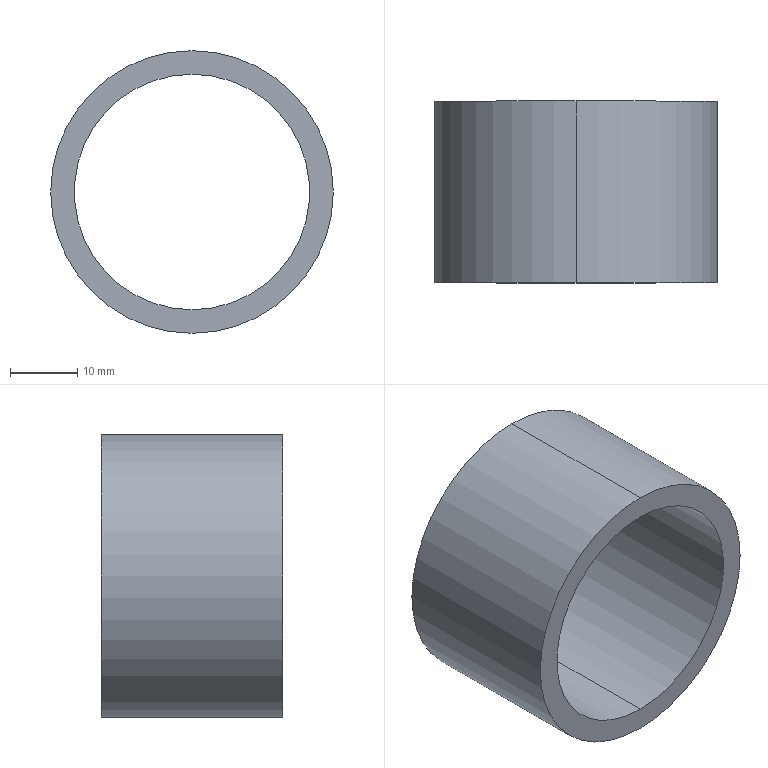Part | STEP file | 01-Spacer 1 | 1 solid | 6 faces | box 42 x 27 x 42 mm | volume 11430 mm3 | cylinder 4 | plane 2 | commonest cylinder face diameters 35 x2 42 x2
STEP:
#1=CARTESIAN_POINT('',(0.,0.,0.));
#2=DIRECTION('',(0.,0.,1.));
#3=DIRECTION('',(1.,0.,0.));
#4=AXIS2_PLACEMENT_3D('',#1,#2,#3);
#5=CARTESIAN_POINT('',(0.,27.,-17.5));
#6=VERTEX_POINT('',#5);
#7=CARTESIAN_POINT('',(0.,0.,-17.5));
#8=VERTEX_POINT('',#7);
#9=CARTESIAN_POINT('',(0.,27.,-17.5));
#10=DIRECTION('',(0.,-1.,0.));
#11=VECTOR('',#10,1.);
#12=LINE('',#9,#11);
#13=CARTESIAN_POINT('',(0.,27.,0.));
#14=DIRECTION('',(0.,-1.,0.));
#15=DIRECTION('',(0.,0.,-1.));
#16=AXIS2_PLACEMENT_3D('',#13,#14,#15);
#17=CYLINDRICAL_SURFACE('',#16,17.5);
#18=CARTESIAN_POINT('',(6.283,0.));
#19=DIRECTION('',(0.,1.));
#20=VECTOR('',#19,1.);
#21=LINE('',#18,#20);
#22=(GEOMETRIC_REPRESENTATION_CONTEXT(2)PARAMETRIC_REPRESENTATION_CONTEXT()REPRESENTATION_CONTEXT('',''));
#23=DEFINITIONAL_REPRESENTATION('',(#21),#22);
#24=PCURVE('',#17,#23);
#25=CARTESIAN_POINT('',(0.,27.,0.));
#26=DIRECTION('',(0.,-1.,0.));
#27=DIRECTION('',(0.,0.,-1.));
#28=AXIS2_PLACEMENT_3D('',#25,#26,#27);
#29=CYLINDRICAL_SURFACE('',#28,17.5);
#30=CARTESIAN_POINT('',(0.,0.));
#31=DIRECTION('',(0.,1.));
#32=VECTOR('',#31,1.);
#33=LINE('',#30,#32);
#34=(GEOMETRIC_REPRESENTATION_CONTEXT(2)PARAMETRIC_REPRESENTATION_CONTEXT()REPRESENTATION_CONTEXT('',''));
#35=DEFINITIONAL_REPRESENTATION('',(#33),#34);
#36=PCURVE('',#29,#35);
#37=SURFACE_CURVE('',#12,(#24,#36),.PCURVE_S1.);
#38=EDGE_CURVE('',#6,#8,#37,.T.);
#39=ORIENTED_EDGE('',*,*,#38,.T.);
#40=CARTESIAN_POINT('',(0.,0.,17.5));
#41=VERTEX_POINT('',#40);
#42=CARTESIAN_POINT('',(0.,0.,0.));
#43=DIRECTION('',(0.,1.,0.));
#44=DIRECTION('',(0.,0.,1.));
#45=AXIS2_PLACEMENT_3D('',#42,#43,#44);
#46=CIRCLE('',#45,17.5);
#47=CARTESIAN_POINT('',(9.425,27.));
#48=DIRECTION('',(-1.,0.));
#49=VECTOR('',#48,1.);
#50=LINE('',#47,#49);
#51=(GEOMETRIC_REPRESENTATION_CONTEXT(2)PARAMETRIC_REPRESENTATION_CONTEXT()REPRESENTATION_CONTEXT('',''));
#52=DEFINITIONAL_REPRESENTATION('',(#50),#51);
#53=PCURVE('',#17,#52);
#54=CARTESIAN_POINT('',(0.,0.,0.));
#55=DIRECTION('',(0.,1.,0.));
#56=DIRECTION('',(0.,0.,1.));
#57=AXIS2_PLACEMENT_3D('',#54,#55,#56);
#58=PLANE('',#57);
#59=CARTESIAN_POINT('',(0.,0.));
#60=DIRECTION('',(1.,0.));
#61=AXIS2_PLACEMENT_2D('',#59,#60);
#62=CIRCLE('',#61,17.5);
#63=(GEOMETRIC_REPRESENTATION_CONTEXT(2)PARAMETRIC_REPRESENTATION_CONTEXT()REPRESENTATION_CONTEXT('',''));
#64=DEFINITIONAL_REPRESENTATION('',(#62),#63);
#65=PCURVE('',#58,#64);
#66=SURFACE_CURVE('',#46,(#53,#65),.PCURVE_S1.);
#67=EDGE_CURVE('',#8,#41,#66,.T.);
#68=ORIENTED_EDGE('',*,*,#67,.T.);
#69=CARTESIAN_POINT('',(0.,27.,17.5));
#70=VERTEX_POINT('',#69);
#71=CARTESIAN_POINT('',(0.,27.,17.5));
#72=DIRECTION('',(0.,-1.,0.));
#73=VECTOR('',#72,1.);
#74=LINE('',#71,#73);
#75=CARTESIAN_POINT('',(3.142,0.));
#76=DIRECTION('',(0.,1.));
#77=VECTOR('',#76,1.);
#78=LINE('',#75,#77);
#79=(GEOMETRIC_REPRESENTATION_CONTEXT(2)PARAMETRIC_REPRESENTATION_CONTEXT()REPRESENTATION_CONTEXT('',''));
#80=DEFINITIONAL_REPRESENTATION('',(#78),#79);
#81=PCURVE('',#17,#80);
#82=CARTESIAN_POINT('',(3.142,0.));
#83=DIRECTION('',(0.,1.));
#84=VECTOR('',#83,1.);
#85=LINE('',#82,#84);
#86=(GEOMETRIC_REPRESENTATION_CONTEXT(2)PARAMETRIC_REPRESENTATION_CONTEXT()REPRESENTATION_CONTEXT('',''));
#87=DEFINITIONAL_REPRESENTATION('',(#85),#86);
#88=PCURVE('',#29,#87);
#89=SURFACE_CURVE('',#74,(#81,#88),.PCURVE_S1.);
#90=EDGE_CURVE('',#70,#41,#89,.T.);
#91=ORIENTED_EDGE('',*,*,#90,.F.);
#92=CARTESIAN_POINT('',(0.,27.,0.));
#93=DIRECTION('',(0.,1.,0.));
#94=DIRECTION('',(0.,0.,1.));
#95=AXIS2_PLACEMENT_3D('',#92,#93,#94);
#96=CIRCLE('',#95,17.5);
#97=CARTESIAN_POINT('',(9.425,0.));
#98=DIRECTION('',(-1.,0.));
#99=VECTOR('',#98,1.);
#100=LINE('',#97,#99);
#101=(GEOMETRIC_REPRESENTATION_CONTEXT(2)PARAMETRIC_REPRESENTATION_CONTEXT()REPRESENTATION_CONTEXT('',''));
#102=DEFINITIONAL_REPRESENTATION('',(#100),#101);
#103=PCURVE('',#17,#102);
#104=CARTESIAN_POINT('',(0.,27.,0.));
#105=DIRECTION('',(0.,1.,0.));
#106=DIRECTION('',(0.,0.,1.));
#107=AXIS2_PLACEMENT_3D('',#104,#105,#106);
#108=PLANE('',#107);
#109=CARTESIAN_POINT('',(0.,0.));
#110=DIRECTION('',(1.,0.));
#111=AXIS2_PLACEMENT_2D('',#109,#110);
#112=CIRCLE('',#111,17.5);
#113=(GEOMETRIC_REPRESENTATION_CONTEXT(2)PARAMETRIC_REPRESENTATION_CONTEXT()REPRESENTATION_CONTEXT('',''));
#114=DEFINITIONAL_REPRESENTATION('',(#112),#113);
#115=PCURVE('',#108,#114);
#116=SURFACE_CURVE('',#96,(#103,#115),.PCURVE_S1.);
#117=EDGE_CURVE('',#6,#70,#116,.T.);
#118=ORIENTED_EDGE('',*,*,#117,.F.);
#119=EDGE_LOOP('',(#39,#68,#91,#118));
#120=FACE_BOUND('',#119,.F.);
#121=ADVANCED_FACE('',(#120),#17,.F.);
#122=CARTESIAN_POINT('',(0.,27.,21.));
#123=VERTEX_POINT('',#122);
#124=CARTESIAN_POINT('',(0.,27.,-21.));
#125=VERTEX_POINT('',#124);
#126=CARTESIAN_POINT('',(0.,27.,0.));
#127=DIRECTION('',(0.,1.,0.));
#128=DIRECTION('',(0.,0.,1.));
#129=AXIS2_PLACEMENT_3D('',#126,#127,#128);
#130=CIRCLE('',#129,21.);
#131=CARTESIAN_POINT('',(0.,27.,0.));
#132=DIRECTION('',(0.,-1.,0.));
#133=DIRECTION('',(0.,0.,-1.));
#134=AXIS2_PLACEMENT_3D('',#131,#132,#133);
#135=CYLINDRICAL_SURFACE('',#134,21.);
#136=CARTESIAN_POINT('',(3.142,0.));
#137=DIRECTION('',(-1.,0.));
#138=VECTOR('',#137,1.);
#139=LINE('',#136,#138);
#140=(GEOMETRIC_REPRESENTATION_CONTEXT(2)PARAMETRIC_REPRESENTATION_CONTEXT()REPRESENTATION_CONTEXT('',''));
#141=DEFINITIONAL_REPRESENTATION('',(#139),#140);
#142=PCURVE('',#135,#141);
#143=CARTESIAN_POINT('',(0.,0.));
#144=DIRECTION('',(1.,0.));
#145=AXIS2_PLACEMENT_2D('',#143,#144);
#146=CIRCLE('',#145,21.);
#147=(GEOMETRIC_REPRESENTATION_CONTEXT(2)PARAMETRIC_REPRESENTATION_CONTEXT()REPRESENTATION_CONTEXT('',''));
#148=DEFINITIONAL_REPRESENTATION('',(#146),#147);
#149=PCURVE('',#108,#148);
#150=SURFACE_CURVE('',#130,(#142,#149),.PCURVE_S1.);
#151=EDGE_CURVE('',#123,#125,#150,.T.);
#152=ORIENTED_EDGE('',*,*,#151,.F.);
#153=CARTESIAN_POINT('',(0.,0.,21.));
#154=VERTEX_POINT('',#153);
#155=CARTESIAN_POINT('',(0.,27.,21.));
#156=DIRECTION('',(0.,-1.,0.));
#157=VECTOR('',#156,1.);
#158=LINE('',#155,#157);
#159=CARTESIAN_POINT('',(3.142,0.));
#160=DIRECTION('',(0.,1.));
#161=VECTOR('',#160,1.);
#162=LINE('',#159,#161);
#163=(GEOMETRIC_REPRESENTATION_CONTEXT(2)PARAMETRIC_REPRESENTATION_CONTEXT()REPRESENTATION_CONTEXT('',''));
#164=DEFINITIONAL_REPRESENTATION('',(#162),#163);
#165=PCURVE('',#135,#164);
#166=CARTESIAN_POINT('',(0.,27.,0.));
#167=DIRECTION('',(0.,-1.,0.));
#168=DIRECTION('',(0.,0.,-1.));
#169=AXIS2_PLACEMENT_3D('',#166,#167,#168);
#170=CYLINDRICAL_SURFACE('',#169,21.);
#171=CARTESIAN_POINT('',(3.142,0.));
#172=DIRECTION('',(0.,1.));
#173=VECTOR('',#172,1.);
#174=LINE('',#171,#173);
#175=(GEOMETRIC_REPRESENTATION_CONTEXT(2)PARAMETRIC_REPRESENTATION_CONTEXT()REPRESENTATION_CONTEXT('',''));
#176=DEFINITIONAL_REPRESENTATION('',(#174),#175);
#177=PCURVE('',#170,#176);
#178=SURFACE_CURVE('',#158,(#165,#177),.PCURVE_S1.);
#179=EDGE_CURVE('',#123,#154,#178,.T.);
#180=ORIENTED_EDGE('',*,*,#179,.T.);
#181=CARTESIAN_POINT('',(0.,0.,-21.));
#182=VERTEX_POINT('',#181);
#183=CARTESIAN_POINT('',(0.,0.,0.));
#184=DIRECTION('',(0.,1.,0.));
#185=DIRECTION('',(0.,0.,1.));
#186=AXIS2_PLACEMENT_3D('',#183,#184,#185);
#187=CIRCLE('',#186,21.);
#188=CARTESIAN_POINT('',(3.142,27.));
#189=DIRECTION('',(-1.,0.));
#190=VECTOR('',#189,1.);
#191=LINE('',#188,#190);
#192=(GEOMETRIC_REPRESENTATION_CONTEXT(2)PARAMETRIC_REPRESENTATION_CONTEXT()REPRESENTATION_CONTEXT('',''));
#193=DEFINITIONAL_REPRESENTATION('',(#191),#192);
#194=PCURVE('',#135,#193);
#195=CARTESIAN_POINT('',(0.,0.));
#196=DIRECTION('',(1.,0.));
#197=AXIS2_PLACEMENT_2D('',#195,#196);
#198=CIRCLE('',#197,21.);
#199=(GEOMETRIC_REPRESENTATION_CONTEXT(2)PARAMETRIC_REPRESENTATION_CONTEXT()REPRESENTATION_CONTEXT('',''));
#200=DEFINITIONAL_REPRESENTATION('',(#198),#199);
#201=PCURVE('',#58,#200);
#202=SURFACE_CURVE('',#187,(#194,#201),.PCURVE_S1.);
#203=EDGE_CURVE('',#154,#182,#202,.T.);
#204=ORIENTED_EDGE('',*,*,#203,.T.);
#205=CARTESIAN_POINT('',(0.,27.,-21.));
#206=DIRECTION('',(0.,-1.,0.));
#207=VECTOR('',#206,1.);
#208=LINE('',#205,#207);
#209=CARTESIAN_POINT('',(0.,0.));
#210=DIRECTION('',(0.,1.));
#211=VECTOR('',#210,1.);
#212=LINE('',#209,#211);
#213=(GEOMETRIC_REPRESENTATION_CONTEXT(2)PARAMETRIC_REPRESENTATION_CONTEXT()REPRESENTATION_CONTEXT('',''));
#214=DEFINITIONAL_REPRESENTATION('',(#212),#213);
#215=PCURVE('',#135,#214);
#216=CARTESIAN_POINT('',(6.283,0.));
#217=DIRECTION('',(0.,1.));
#218=VECTOR('',#217,1.);
#219=LINE('',#216,#218);
#220=(GEOMETRIC_REPRESENTATION_CONTEXT(2)PARAMETRIC_REPRESENTATION_CONTEXT()REPRESENTATION_CONTEXT('',''));
#221=DEFINITIONAL_REPRESENTATION('',(#219),#220);
#222=PCURVE('',#170,#221);
#223=SURFACE_CURVE('',#208,(#215,#222),.PCURVE_S1.);
#224=EDGE_CURVE('',#125,#182,#223,.T.);
#225=ORIENTED_EDGE('',*,*,#224,.F.);
#226=EDGE_LOOP('',(#152,#180,#204,#225));
#227=FACE_BOUND('',#226,.T.);
#228=ADVANCED_FACE('',(#227),#135,.T.);
#229=CARTESIAN_POINT('',(0.,27.,0.));
#230=DIRECTION('',(0.,1.,0.));
#231=DIRECTION('',(0.,0.,1.));
#232=AXIS2_PLACEMENT_3D('',#229,#230,#231);
#233=CIRCLE('',#232,21.);
#234=CARTESIAN_POINT('',(0.,0.));
#235=DIRECTION('',(1.,0.));
#236=AXIS2_PLACEMENT_2D('',#234,#235);
#237=CIRCLE('',#236,21.);
#238=(GEOMETRIC_REPRESENTATION_CONTEXT(2)PARAMETRIC_REPRESENTATION_CONTEXT()REPRESENTATION_CONTEXT('',''));
#239=DEFINITIONAL_REPRESENTATION('',(#237),#238);
#240=PCURVE('',#108,#239);
#241=CARTESIAN_POINT('',(9.425,0.));
#242=DIRECTION('',(-1.,0.));
#243=VECTOR('',#242,1.);
#244=LINE('',#241,#243);
#245=(GEOMETRIC_REPRESENTATION_CONTEXT(2)PARAMETRIC_REPRESENTATION_CONTEXT()REPRESENTATION_CONTEXT('',''));
#246=DEFINITIONAL_REPRESENTATION('',(#244),#245);
#247=PCURVE('',#170,#246);
#248=SURFACE_CURVE('',#233,(#240,#247),.PCURVE_S1.);
#249=EDGE_CURVE('',#125,#123,#248,.T.);
#250=ORIENTED_EDGE('',*,*,#249,.T.);
#251=ORIENTED_EDGE('',*,*,#151,.T.);
#252=EDGE_LOOP('',(#250,#251));
#253=FACE_BOUND('',#252,.T.);
#254=ORIENTED_EDGE('',*,*,#117,.F.);
#255=CARTESIAN_POINT('',(0.,27.,0.));
#256=DIRECTION('',(0.,1.,0.));
#257=DIRECTION('',(0.,0.,1.));
#258=AXIS2_PLACEMENT_3D('',#255,#256,#257);
#259=CIRCLE('',#258,17.5);
#260=CARTESIAN_POINT('',(0.,0.));
#261=DIRECTION('',(1.,0.));
#262=AXIS2_PLACEMENT_2D('',#260,#261);
#263=CIRCLE('',#262,17.5);
#264=(GEOMETRIC_REPRESENTATION_CONTEXT(2)PARAMETRIC_REPRESENTATION_CONTEXT()REPRESENTATION_CONTEXT('',''));
#265=DEFINITIONAL_REPRESENTATION('',(#263),#264);
#266=PCURVE('',#108,#265);
#267=CARTESIAN_POINT('',(3.142,0.));
#268=DIRECTION('',(-1.,0.));
#269=VECTOR('',#268,1.);
#270=LINE('',#267,#269);
#271=(GEOMETRIC_REPRESENTATION_CONTEXT(2)PARAMETRIC_REPRESENTATION_CONTEXT()REPRESENTATION_CONTEXT('',''));
#272=DEFINITIONAL_REPRESENTATION('',(#270),#271);
#273=PCURVE('',#29,#272);
#274=SURFACE_CURVE('',#259,(#266,#273),.PCURVE_S1.);
#275=EDGE_CURVE('',#70,#6,#274,.T.);
#276=ORIENTED_EDGE('',*,*,#275,.F.);
#277=EDGE_LOOP('',(#254,#276));
#278=FACE_BOUND('',#277,.T.);
#279=ADVANCED_FACE('',(#253,#278),#108,.T.);
#280=CARTESIAN_POINT('',(0.,0.,0.));
#281=DIRECTION('',(0.,1.,0.));
#282=DIRECTION('',(0.,0.,1.));
#283=AXIS2_PLACEMENT_3D('',#280,#281,#282);
#284=CIRCLE('',#283,21.);
#285=CARTESIAN_POINT('',(0.,0.));
#286=DIRECTION('',(1.,0.));
#287=AXIS2_PLACEMENT_2D('',#285,#286);
#288=CIRCLE('',#287,21.);
#289=(GEOMETRIC_REPRESENTATION_CONTEXT(2)PARAMETRIC_REPRESENTATION_CONTEXT()REPRESENTATION_CONTEXT('',''));
#290=DEFINITIONAL_REPRESENTATION('',(#288),#289);
#291=PCURVE('',#58,#290);
#292=CARTESIAN_POINT('',(9.425,27.));
#293=DIRECTION('',(-1.,0.));
#294=VECTOR('',#293,1.);
#295=LINE('',#292,#294);
#296=(GEOMETRIC_REPRESENTATION_CONTEXT(2)PARAMETRIC_REPRESENTATION_CONTEXT()REPRESENTATION_CONTEXT('',''));
#297=DEFINITIONAL_REPRESENTATION('',(#295),#296);
#298=PCURVE('',#170,#297);
#299=SURFACE_CURVE('',#284,(#291,#298),.PCURVE_S1.);
#300=EDGE_CURVE('',#182,#154,#299,.T.);
#301=ORIENTED_EDGE('',*,*,#300,.F.);
#302=ORIENTED_EDGE('',*,*,#203,.F.);
#303=EDGE_LOOP('',(#301,#302));
#304=FACE_BOUND('',#303,.T.);
#305=ORIENTED_EDGE('',*,*,#67,.T.);
#306=CARTESIAN_POINT('',(0.,0.,0.));
#307=DIRECTION('',(0.,1.,0.));
#308=DIRECTION('',(0.,0.,1.));
#309=AXIS2_PLACEMENT_3D('',#306,#307,#308);
#310=CIRCLE('',#309,17.5);
#311=CARTESIAN_POINT('',(0.,0.));
#312=DIRECTION('',(1.,0.));
#313=AXIS2_PLACEMENT_2D('',#311,#312);
#314=CIRCLE('',#313,17.5);
#315=(GEOMETRIC_REPRESENTATION_CONTEXT(2)PARAMETRIC_REPRESENTATION_CONTEXT()REPRESENTATION_CONTEXT('',''));
#316=DEFINITIONAL_REPRESENTATION('',(#314),#315);
#317=PCURVE('',#58,#316);
#318=CARTESIAN_POINT('',(3.142,27.));
#319=DIRECTION('',(-1.,0.));
#320=VECTOR('',#319,1.);
#321=LINE('',#318,#320);
#322=(GEOMETRIC_REPRESENTATION_CONTEXT(2)PARAMETRIC_REPRESENTATION_CONTEXT()REPRESENTATION_CONTEXT('',''));
#323=DEFINITIONAL_REPRESENTATION('',(#321),#322);
#324=PCURVE('',#29,#323);
#325=SURFACE_CURVE('',#310,(#317,#324),.PCURVE_S1.);
#326=EDGE_CURVE('',#41,#8,#325,.T.);
#327=ORIENTED_EDGE('',*,*,#326,.T.);
#328=EDGE_LOOP('',(#305,#327));
#329=FACE_BOUND('',#328,.T.);
#330=ADVANCED_FACE('',(#304,#329),#58,.F.);
#331=ORIENTED_EDGE('',*,*,#179,.F.);
#332=ORIENTED_EDGE('',*,*,#249,.F.);
#333=ORIENTED_EDGE('',*,*,#224,.T.);
#334=ORIENTED_EDGE('',*,*,#300,.T.);
#335=EDGE_LOOP('',(#331,#332,#333,#334));
#336=FACE_BOUND('',#335,.T.);
#337=ADVANCED_FACE('',(#336),#170,.T.);
#338=ORIENTED_EDGE('',*,*,#326,.T.);
#339=ORIENTED_EDGE('',*,*,#38,.F.);
#340=ORIENTED_EDGE('',*,*,#275,.F.);
#341=ORIENTED_EDGE('',*,*,#90,.T.);
#342=EDGE_LOOP('',(#338,#339,#340,#341));
#343=FACE_BOUND('',#342,.F.);
#344=ADVANCED_FACE('',(#343),#29,.F.);
#345=CLOSED_SHELL('',(#121,#228,#279,#330,#337,#344));
#346=MANIFOLD_SOLID_BREP('',#345);
#347=(LENGTH_UNIT()NAMED_UNIT(*)SI_UNIT(.MILLI.,.METRE.));
#348=UNCERTAINTY_MEASURE_WITH_UNIT(LENGTH_MEASURE(0.0000001),#347,'','');
#349=(NAMED_UNIT(*)PLANE_ANGLE_UNIT()SI_UNIT($,.RADIAN.));
#350=(NAMED_UNIT(*)SI_UNIT($,.STERADIAN.)SOLID_ANGLE_UNIT());
#351=(GEOMETRIC_REPRESENTATION_CONTEXT(3)GLOBAL_UNCERTAINTY_ASSIGNED_CONTEXT((#348))GLOBAL_UNIT_ASSIGNED_CONTEXT((#347,#349,#350))REPRESENTATION_CONTEXT('',''));
#352=ADVANCED_BREP_SHAPE_REPRESENTATION('',(#4,#346),#351);